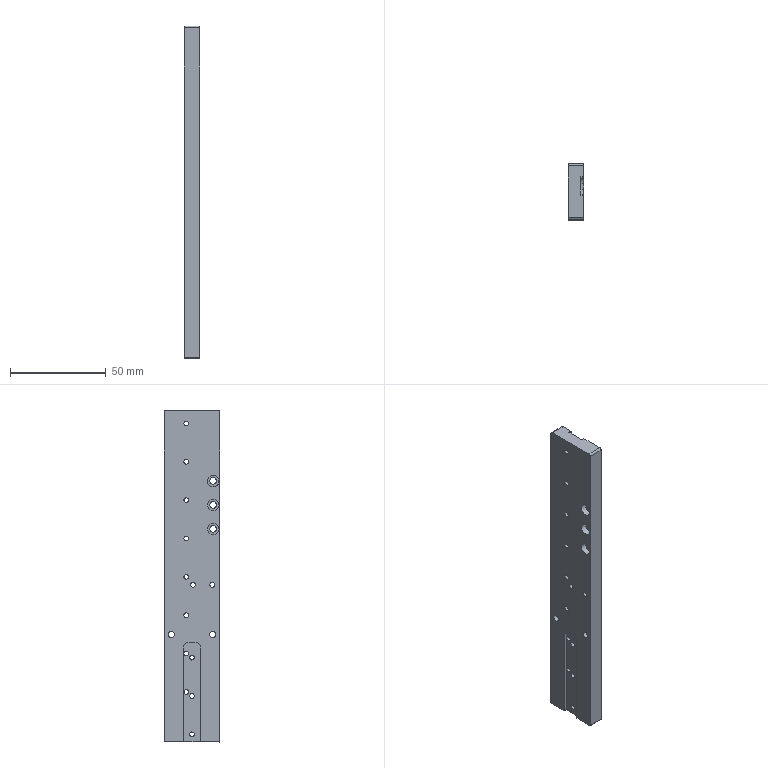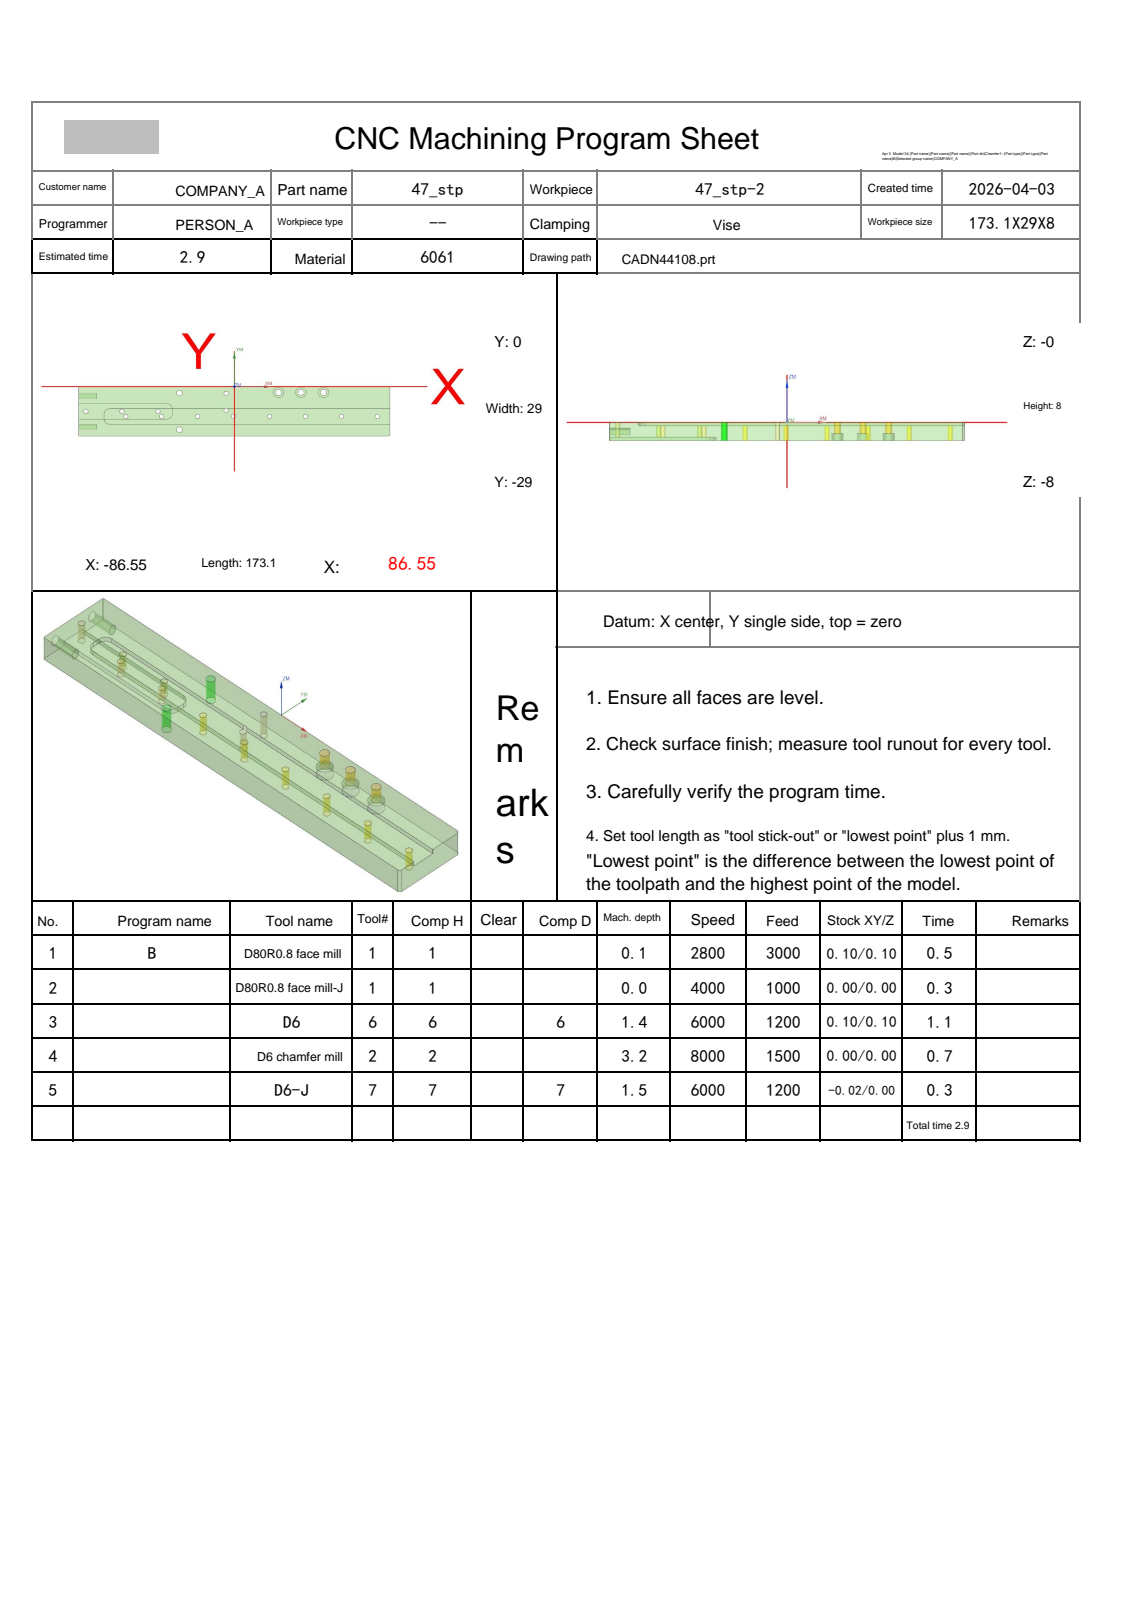NC program | NX | posted by the shop | part box 8 x 29 x 173.1 mm
Whole program:
%
O0001
(Machine time: 3.81 MIN)
(===Total Tool:4===)
(T1=D80R0.8 face mill D=80.  R=0.8  D-  H01 Z=-0.   )
(T6=D6      D=6.   R=0.   D6  H06 Z=-1.4  )
(T2=D6 chamfer mill   D=6.   R=0.   D-  H02 Z=-3.25 )
(T7=D6-J    D=6.   R=0.   D7  H07 Z=-1.5  )
G80 G90 G17 G49 G40
G91 G28 Z0
M01
N1 T01 M06
(D80R0.8 face mill  D=80. R=0.8 H=01 ce=0.10 di=0.10)
G00 G90 G54 X138.647 Y-14.5 M03 S2800
G43 H01 Z20.
M08
Z3.525
G01 Z1.525 F3000.
X126.647
X-126.647
X-138.647
Z3.525
G00 X138.647
Z3.05
G01 Z1.05
X126.647
X-126.647
X-138.647
Z3.05
G00 X138.647
Z2.575
G01 Z.575
X126.647
X-126.647
X-138.647
Z2.575
G00 X138.647
Z2.1
G01 Z.1
X126.647
X-126.647
X-138.647
Z2.1
G00 Z20.
G91 G28 Z0.0
M05
M09
G91 G28 Z0.0
M01
N2 T01 M06
(D80R0.8 face mill-J  D=80. R=0.8 H=01 ce=0.00 di=0.00)
G00 G90 G54 X138.549 Y-14.5 M03 S4000
G43 H01 Z20.
M08
Z2.
G01 Z0.0 F1000.
X126.549
X-126.549
X-138.549
Z2.
G00 Z20.
G91 G28 Z0.0
M05
M09
G91 G28 Z0.0
M01
N3 T06 M06
(D6  D=6. R=0. H=06 ce=0.10 di=0.10)
G00 G90 G54 X90.746 Y-13.829 M03 S6000
G43 H06 Z20.
M08
Z.15
G01 Z-.35 F1200.
G41 D06
X90.65 Y-13.8
G03 X90.357 Y-13.756 I-.293 J-.956
X89.65 Y-14.049 I0.0 J-1.
G01 X87.634 Y-16.065
X-3.805
G02 X-4.574 Y-15.968 I0.0 J3.1
X-5.344 Y-16.065 I-.77 J3.003
G01 X-69.385
Y-18.935
X87.634
X89.65 Y-20.951
G03 X90.357 Y-21.244 I.707 J.707
X90.65 Y-21.2 I0.0 J1.
G01 G40 X90.746 Y-21.171
Z.15
G00 Z20.
Y-13.829
Z-.2
G01 Z-.7
G41 D06
X90.65 Y-13.8
G03 X90.357 Y-13.756 I-.293 J-.956
X89.65 Y-14.049 I0.0 J-1.
G01 X87.634 Y-16.065
X-3.805
G02 X-4.574 Y-15.968 I0.0 J3.1
X-5.344 Y-16.065 I-.77 J3.003
G01 X-69.385
Y-18.935
X87.634
X89.65 Y-20.951
G03 X90.357 Y-21.244 I.707 J.707
X90.65 Y-21.2 I0.0 J1.
G01 G40 X90.746 Y-21.171
Z-.2
G00 Z20.
Y-13.829
Z-.55
G01 Z-1.05
G41 D06
X90.65 Y-13.8
G03 X90.357 Y-13.756 I-.293 J-.956
X89.65 Y-14.049 I0.0 J-1.
G01 X87.634 Y-16.065
X-3.805
G02 X-4.574 Y-15.968 I0.0 J3.1
X-5.344 Y-16.065 I-.77 J3.003
G01 X-69.385
Y-18.935
X87.634
X89.65 Y-20.951
G03 X90.357 Y-21.244 I.707 J.707
X90.65 Y-21.2 I0.0 J1.
G01 G40 X90.746 Y-21.171
Z-.55
G00 Z20.
Y-13.829
Z-.9
G01 Z-1.4
G41 D06
X90.65 Y-13.8
G03 X90.357 Y-13.756 I-.293 J-.956
X89.65 Y-14.049 I0.0 J-1.
G01 X87.634 Y-16.065
X-3.805
G02 X-4.574 Y-15.968 I0.0 J3.1
X-5.344 Y-16.065 I-.77 J3.003
G01 X-69.385
Y-18.935
X87.634
X89.65 Y-20.951
G03 X90.357 Y-21.244 I.707 J.707
X90.65 Y-21.2 I0.0 J1.
G01 G40 X90.746 Y-21.171
Z-.9
G00 Z20.
G91 G28 Z0.0
M05
M09
G91 G28 Z0.0
M01
N4 T02 M06
(D6 chamfer mill  D=6. R=0. H=02 ce=0.00 di=0.10)
G00 G90 G54 X-82.55 Y-14.5 M03 S8000
G43 H02 Z20.
M08
G98 G81 X-82.55 Y-14.5 Z-1.75 R3. F1000.
X-60.45 Y-17.5 Z-3.25 R1.5
X-40.45
X-20.45
X-.45
X-4.574 Y-3.95 Z-1.75 R3.
X19.55 Y-17.5 Z-3.25 R1.5
X39.55
X59.55
X79.55
G80
G00 Z20.
G00 G90 X-30.55 Y-3.75 M03 S8000
Z20.
G98 G81 X-30.55 Y-3.75 Z-2.2 R3. F1000.
Y-25.25
G80
G00 Z20.
G00 G90 X49.55 Y-3.455 M03 S8000
Z20.
G98 G81 X49.55 Y-3.455 Z-2.05 R3. F1000.
X37.05
X24.55
G80
G00 Z20.
G00 G90 X-.786 Y1.227 M03 S6500
Z20.
Z.172
G01 Z-1.199 F1500.
G03 X-.5 Y1.027 I1.286 J1.532
G01 X-.454 Y.997
X-.4 Y1.
X85.55
G02 X87.55 Y-1. I0.0 J-2.
G01 Y-12.765
X87.516 Y-13.024
X87.416 Y-13.265
X87.257 Y-13.472
X87.057 Y-13.672
X86.85 Y-13.831
X86.609 Y-13.931
X86.35 Y-13.965
X-3.805
X-4.024 Y-13.941
X-4.233 Y-13.869
X-4.42 Y-13.753
X-4.52 Y-13.706
X-4.629
X-4.728 Y-13.753
X-4.916 Y-13.869
X-5.125 Y-13.941
X-5.344 Y-13.965
X-69.45
G03 X-71.485 Y-16. I0.0 J-2.035
G01 Y-19.
G03 X-69.45 Y-21.035 I2.035 J0.0
G01 X86.35
X86.609 Y-21.069
X86.85 Y-21.169
X87.057 Y-21.328
X87.257 Y-21.528
X87.416 Y-21.735
X87.516 Y-21.976
X87.55 Y-22.235
Y-28.
G02 X85.55 Y-30. I-2. J0.0
G01 X-86.35
X-86.609 Y-29.966
X-86.85 Y-29.866
X-87.057 Y-29.707
X-87.257 Y-29.507
X-87.416 Y-29.3
X-87.516 Y-29.059
X-87.55 Y-28.8
Y-.2
X-87.516 Y.059
X-87.416 Y.3
X-87.257 Y.507
X-87.057 Y.707
X-86.85 Y.866
X-86.609 Y.966
X-86.35 Y1.
X-.4
X-.346 Y.997
X-.3 Y1.027
G03 X-.014 Y1.227 I-1. J1.732
G01 Z.172
G00 Z10.
X-31.044 Y-24.831
Z.405
G01 Z-1.199
G03 X-31.191 Y-25.147 I1.732 J-1.
G01 X-31.212 Y-25.197
X-31.2 Y-25.25
G03 X-30.55 Y-25.9 I.65 J0.0
X-29.9 Y-25.25 I0.0 J.65
X-30.55 Y-24.6 I-.65 J0.0
X-31.2 Y-25.25 I0.0 J-.65
G01 X-31.212 Y-25.303
X-31.191 Y-25.353
G03 X-31.044 Y-25.669 I1.879 J.684
G01 Z.405
G00 Z10.
Y-3.331
Z.405
G01 Z-1.199
G03 X-31.191 Y-3.647 I1.732 J-1.
G01 X-31.212 Y-3.697
X-31.2 Y-3.75
G03 X-30.55 Y-4.4 I.65 J0.0
X-29.9 Y-3.75 I0.0 J.65
X-30.55 Y-3.1 I-.65 J0.0
X-31.2 Y-3.75 I0.0 J-.65
G01 X-31.212 Y-3.803
X-31.191 Y-3.853
G03 X-31.044 Y-4.169 I1.879 J.684
G01 Z.405
G00 Z10.
X23.974 Y-3.043
Z.363
G01 Z-1.199
G03 X23.814 Y-3.352 I1.687 J-1.075
G01 X23.79 Y-3.401
X23.8 Y-3.455
G03 X24.55 Y-4.205 I.75 J0.0
X25.3 Y-3.455 I0.0 J.75
X24.55 Y-2.705 I-.75 J0.0
X23.826 Y-3.261 I0.0 J-.75
G01 X23.8 Y-3.455
X23.79 Y-3.509
X23.814 Y-3.558
G03 X23.974 Y-3.867 I1.848 J.765
G01 Z.363
G00 Z10.
X36.474 Y-3.043
Z.363
G01 Z-1.199
G03 X36.314 Y-3.352 I1.687 J-1.075
G01 X36.29 Y-3.401
X36.3 Y-3.455
G03 X37.05 Y-4.205 I.75 J0.0
X37.8 Y-3.455 I0.0 J.75
X37.05 Y-2.705 I-.75 J0.0
X36.326 Y-3.261 I0.0 J-.75
G01 X36.3 Y-3.455
X36.29 Y-3.509
X36.314 Y-3.558
G03 X36.474 Y-3.867 I1.848 J.765
G01 Z.363
G00 Z10.
X48.974 Y-3.043
Z.363
G01 Z-1.199
G03 X48.814 Y-3.352 I1.687 J-1.075
G01 X48.79 Y-3.401
X48.8 Y-3.455
G03 X49.55 Y-4.205 I.75 J0.0
X50.3 Y-3.455 I0.0 J.75
X49.55 Y-2.705 I-.75 J0.0
X48.826 Y-3.261 I0.0 J-.75
G01 X48.8 Y-3.455
X48.79 Y-3.509
X48.814 Y-3.558
G03 X48.974 Y-3.867 I1.848 J.765
G01 Z.363
G00 Z10.
X87.55 Y-15.354
Z1.301
G01 Z-2.699
Y-19.646
Z1.301
G00 Z20.
G91 G28 Z0.0
M05
M09
G91 G28 Z0.0
M01
N5 T07 M06
(D6-J  D=6. R=0. H=07 ce=-0.02 di=0.00)
G00 G90 G54 X90.63 Y-10.927 M03 S6000
G43 H07 Z20.
M08
Z-1.
G01 Z-1.5 F1200.
G41 D07
X90.53
G03 X89.53 Y-11.927 I0.0 J-1.
G01 Y-13.999
X87.584 Y-15.945
X-3.805
G02 X-4.574 Y-15.844 I0.0 J2.98
X-5.344 Y-15.945 I-.77 J2.879
G01 X-69.45
X-69.483 Y-15.944
X-69.506 Y-15.968
X-69.505 Y-16.
Y-19.
X-69.506 Y-19.033
X-69.483 Y-19.056
X-69.45 Y-19.055
X87.584
X89.53 Y-21.001
Y-23.073
G03 X90.53 Y-24.073 I1. J0.0
G01 G40 X90.63
Z-1.
G00 Z20.
M05
M09
G91 G28 Z0.0
G91 G28 Y0.0
M30
%